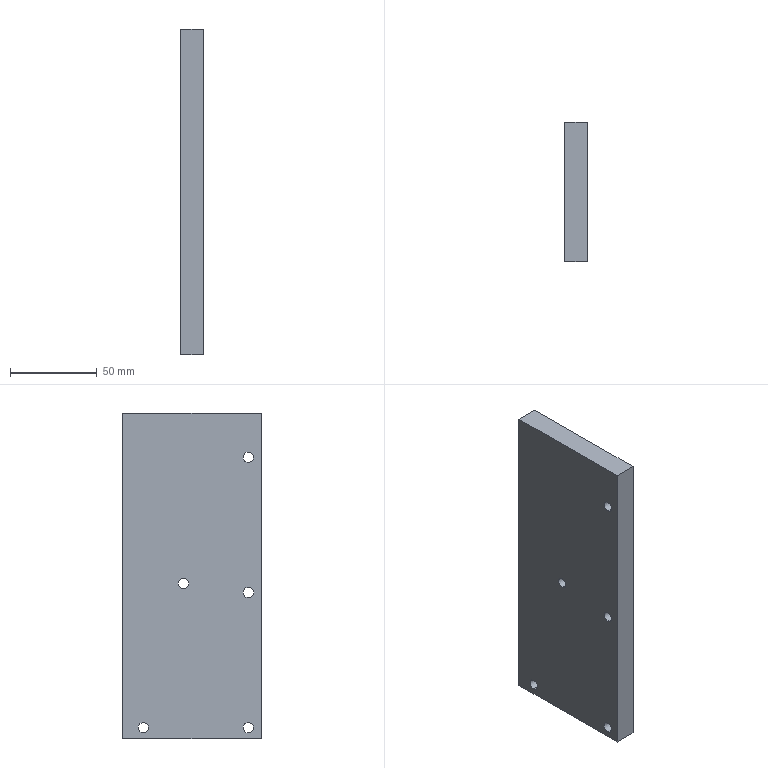Part | SolidWorks | features Cut 6, Extrusion 1 | 1 solid | 31 faces | box 13 x 80 x 188 mm | volume 192174 mm3 | cylinder 20 | plane 11 | commonest cylinder face diameters 6 x10 10 x10
STEP:
#1=CARTESIAN_POINT('',(0.,28.,-84.5));
#2=VERTEX_POINT('',#1);
#3=CARTESIAN_POINT('',(0.,28.,-90.5));
#4=VERTEX_POINT('',#3);
#5=CARTESIAN_POINT('',(0.,28.,-87.5));
#6=DIRECTION('',(1.,0.,0.));
#7=DIRECTION('',(0.,0.,1.));
#8=AXIS2_PLACEMENT_3D('',#5,#6,#7);
#9=CIRCLE('',#8,3.);
#10=EDGE_CURVE('',#2,#4,#9,.T.);
#11=ORIENTED_EDGE('',*,*,#10,.F.);
#12=CARTESIAN_POINT('',(7.,28.,-84.5));
#13=VERTEX_POINT('',#12);
#14=CARTESIAN_POINT('',(-0.001,28.,-84.5));
#15=DIRECTION('',(1.,0.,0.));
#16=VECTOR('',#15,1000.);
#17=LINE('',#14,#16);
#18=EDGE_CURVE('',#2,#13,#17,.T.);
#19=ORIENTED_EDGE('',*,*,#18,.T.);
#20=CARTESIAN_POINT('',(7.,28.,-90.5));
#21=VERTEX_POINT('',#20);
#22=CARTESIAN_POINT('',(7.,28.,-87.5));
#23=DIRECTION('',(-1.,0.,0.));
#24=DIRECTION('',(0.,0.,-1.));
#25=AXIS2_PLACEMENT_3D('',#22,#23,#24);
#26=CIRCLE('',#25,3.);
#27=EDGE_CURVE('',#21,#13,#26,.T.);
#28=ORIENTED_EDGE('',*,*,#27,.F.);
#29=CARTESIAN_POINT('',(-0.001,28.,-90.5));
#30=DIRECTION('',(1.,0.,0.));
#31=VECTOR('',#30,1000.);
#32=LINE('',#29,#31);
#33=EDGE_CURVE('',#4,#21,#32,.T.);
#34=ORIENTED_EDGE('',*,*,#33,.F.);
#35=EDGE_LOOP('',(#11,#19,#28,#34));
#36=FACE_OUTER_BOUND('',#35,.T.);
#37=CARTESIAN_POINT('',(-0.001,28.,-87.5));
#38=DIRECTION('',(1.,0.,0.));
#39=DIRECTION('',(0.,0.,-1.));
#40=AXIS2_PLACEMENT_3D('',#37,#38,#39);
#41=CYLINDRICAL_SURFACE('',#40,3.);
#42=ADVANCED_FACE('',(#36),#41,.F.);
#43=CARTESIAN_POINT('',(7.,28.,-82.5));
#44=VERTEX_POINT('',#43);
#45=CARTESIAN_POINT('',(7.,28.,-92.5));
#46=VERTEX_POINT('',#45);
#47=CARTESIAN_POINT('',(7.,28.,-87.5));
#48=DIRECTION('',(1.,0.,0.));
#49=DIRECTION('',(0.,0.,-1.));
#50=AXIS2_PLACEMENT_3D('',#47,#48,#49);
#51=CIRCLE('',#50,5.);
#52=EDGE_CURVE('',#44,#46,#51,.T.);
#53=ORIENTED_EDGE('',*,*,#52,.F.);
#54=CARTESIAN_POINT('',(13.,28.,-82.5));
#55=VERTEX_POINT('',#54);
#56=CARTESIAN_POINT('',(7.,28.,-82.5));
#57=DIRECTION('',(1.,0.,0.));
#58=VECTOR('',#57,1000.);
#59=LINE('',#56,#58);
#60=EDGE_CURVE('',#44,#55,#59,.T.);
#61=ORIENTED_EDGE('',*,*,#60,.T.);
#62=CARTESIAN_POINT('',(13.,28.,-92.5));
#63=VERTEX_POINT('',#62);
#64=CARTESIAN_POINT('',(13.,28.,-87.5));
#65=DIRECTION('',(1.,0.,0.));
#66=DIRECTION('',(0.,0.,-1.));
#67=AXIS2_PLACEMENT_3D('',#64,#65,#66);
#68=CIRCLE('',#67,5.);
#69=EDGE_CURVE('',#55,#63,#68,.T.);
#70=ORIENTED_EDGE('',*,*,#69,.T.);
#71=CARTESIAN_POINT('',(7.,28.,-92.5));
#72=DIRECTION('',(1.,0.,0.));
#73=VECTOR('',#72,1000.);
#74=LINE('',#71,#73);
#75=EDGE_CURVE('',#46,#63,#74,.T.);
#76=ORIENTED_EDGE('',*,*,#75,.F.);
#77=EDGE_LOOP('',(#53,#61,#70,#76));
#78=FACE_OUTER_BOUND('',#77,.T.);
#79=CARTESIAN_POINT('',(7.,28.,-87.5));
#80=DIRECTION('',(1.,0.,0.));
#81=DIRECTION('',(0.,0.,-1.));
#82=AXIS2_PLACEMENT_3D('',#79,#80,#81);
#83=CYLINDRICAL_SURFACE('',#82,5.);
#84=ADVANCED_FACE('',(#78),#83,.F.);
#85=CARTESIAN_POINT('',(0.,-32.5,-84.5));
#86=VERTEX_POINT('',#85);
#87=CARTESIAN_POINT('',(0.,-32.5,-90.5));
#88=VERTEX_POINT('',#87);
#89=CARTESIAN_POINT('',(0.,-32.5,-87.5));
#90=DIRECTION('',(1.,0.,0.));
#91=DIRECTION('',(0.,0.,1.));
#92=AXIS2_PLACEMENT_3D('',#89,#90,#91);
#93=CIRCLE('',#92,3.);
#94=EDGE_CURVE('',#86,#88,#93,.T.);
#95=ORIENTED_EDGE('',*,*,#94,.F.);
#96=CARTESIAN_POINT('',(7.,-32.5,-84.5));
#97=VERTEX_POINT('',#96);
#98=CARTESIAN_POINT('',(-0.001,-32.5,-84.5));
#99=DIRECTION('',(1.,0.,0.));
#100=VECTOR('',#99,1000.);
#101=LINE('',#98,#100);
#102=EDGE_CURVE('',#86,#97,#101,.T.);
#103=ORIENTED_EDGE('',*,*,#102,.T.);
#104=CARTESIAN_POINT('',(7.,-32.5,-90.5));
#105=VERTEX_POINT('',#104);
#106=CARTESIAN_POINT('',(7.,-32.5,-87.5));
#107=DIRECTION('',(-1.,0.,0.));
#108=DIRECTION('',(0.,0.,-1.));
#109=AXIS2_PLACEMENT_3D('',#106,#107,#108);
#110=CIRCLE('',#109,3.);
#111=EDGE_CURVE('',#105,#97,#110,.T.);
#112=ORIENTED_EDGE('',*,*,#111,.F.);
#113=CARTESIAN_POINT('',(-0.001,-32.5,-90.5));
#114=DIRECTION('',(1.,0.,0.));
#115=VECTOR('',#114,1000.);
#116=LINE('',#113,#115);
#117=EDGE_CURVE('',#88,#105,#116,.T.);
#118=ORIENTED_EDGE('',*,*,#117,.F.);
#119=EDGE_LOOP('',(#95,#103,#112,#118));
#120=FACE_OUTER_BOUND('',#119,.T.);
#121=CARTESIAN_POINT('',(-0.001,-32.5,-87.5));
#122=DIRECTION('',(1.,0.,0.));
#123=DIRECTION('',(0.,0.,-1.));
#124=AXIS2_PLACEMENT_3D('',#121,#122,#123);
#125=CYLINDRICAL_SURFACE('',#124,3.);
#126=ADVANCED_FACE('',(#120),#125,.F.);
#127=CARTESIAN_POINT('',(0.,-32.5,-6.5));
#128=VERTEX_POINT('',#127);
#129=CARTESIAN_POINT('',(0.,-32.5,-12.5));
#130=VERTEX_POINT('',#129);
#131=CARTESIAN_POINT('',(0.,-32.5,-9.5));
#132=DIRECTION('',(1.,0.,0.));
#133=DIRECTION('',(0.,0.,1.));
#134=AXIS2_PLACEMENT_3D('',#131,#132,#133);
#135=CIRCLE('',#134,3.);
#136=EDGE_CURVE('',#128,#130,#135,.T.);
#137=ORIENTED_EDGE('',*,*,#136,.F.);
#138=CARTESIAN_POINT('',(7.,-32.5,-6.5));
#139=VERTEX_POINT('',#138);
#140=CARTESIAN_POINT('',(-0.001,-32.5,-6.5));
#141=DIRECTION('',(1.,0.,0.));
#142=VECTOR('',#141,1000.);
#143=LINE('',#140,#142);
#144=EDGE_CURVE('',#128,#139,#143,.T.);
#145=ORIENTED_EDGE('',*,*,#144,.T.);
#146=CARTESIAN_POINT('',(7.,-32.5,-12.5));
#147=VERTEX_POINT('',#146);
#148=CARTESIAN_POINT('',(7.,-32.5,-9.5));
#149=DIRECTION('',(-1.,0.,0.));
#150=DIRECTION('',(0.,0.,-1.));
#151=AXIS2_PLACEMENT_3D('',#148,#149,#150);
#152=CIRCLE('',#151,3.);
#153=EDGE_CURVE('',#147,#139,#152,.T.);
#154=ORIENTED_EDGE('',*,*,#153,.F.);
#155=CARTESIAN_POINT('',(-0.001,-32.5,-12.5));
#156=DIRECTION('',(1.,0.,0.));
#157=VECTOR('',#156,1000.);
#158=LINE('',#155,#157);
#159=EDGE_CURVE('',#130,#147,#158,.T.);
#160=ORIENTED_EDGE('',*,*,#159,.F.);
#161=EDGE_LOOP('',(#137,#145,#154,#160));
#162=FACE_OUTER_BOUND('',#161,.T.);
#163=CARTESIAN_POINT('',(-0.001,-32.5,-9.5));
#164=DIRECTION('',(1.,0.,0.));
#165=DIRECTION('',(0.,0.,-1.));
#166=AXIS2_PLACEMENT_3D('',#163,#164,#165);
#167=CYLINDRICAL_SURFACE('',#166,3.);
#168=ADVANCED_FACE('',(#162),#167,.F.);
#169=CARTESIAN_POINT('',(0.,-32.5,71.5));
#170=VERTEX_POINT('',#169);
#171=CARTESIAN_POINT('',(0.,-32.5,65.5));
#172=VERTEX_POINT('',#171);
#173=CARTESIAN_POINT('',(0.,-32.5,68.5));
#174=DIRECTION('',(1.,0.,0.));
#175=DIRECTION('',(0.,0.,1.));
#176=AXIS2_PLACEMENT_3D('',#173,#174,#175);
#177=CIRCLE('',#176,3.);
#178=EDGE_CURVE('',#170,#172,#177,.T.);
#179=ORIENTED_EDGE('',*,*,#178,.F.);
#180=CARTESIAN_POINT('',(7.,-32.5,71.5));
#181=VERTEX_POINT('',#180);
#182=CARTESIAN_POINT('',(-0.001,-32.5,71.5));
#183=DIRECTION('',(1.,0.,0.));
#184=VECTOR('',#183,1000.);
#185=LINE('',#182,#184);
#186=EDGE_CURVE('',#170,#181,#185,.T.);
#187=ORIENTED_EDGE('',*,*,#186,.T.);
#188=CARTESIAN_POINT('',(7.,-32.5,65.5));
#189=VERTEX_POINT('',#188);
#190=CARTESIAN_POINT('',(7.,-32.5,68.5));
#191=DIRECTION('',(-1.,0.,0.));
#192=DIRECTION('',(0.,0.,-1.));
#193=AXIS2_PLACEMENT_3D('',#190,#191,#192);
#194=CIRCLE('',#193,3.);
#195=EDGE_CURVE('',#189,#181,#194,.T.);
#196=ORIENTED_EDGE('',*,*,#195,.F.);
#197=CARTESIAN_POINT('',(-0.001,-32.5,65.5));
#198=DIRECTION('',(1.,0.,0.));
#199=VECTOR('',#198,1000.);
#200=LINE('',#197,#199);
#201=EDGE_CURVE('',#172,#189,#200,.T.);
#202=ORIENTED_EDGE('',*,*,#201,.F.);
#203=EDGE_LOOP('',(#179,#187,#196,#202));
#204=FACE_OUTER_BOUND('',#203,.T.);
#205=CARTESIAN_POINT('',(-0.001,-32.5,68.5));
#206=DIRECTION('',(1.,0.,0.));
#207=DIRECTION('',(0.,0.,-1.));
#208=AXIS2_PLACEMENT_3D('',#205,#206,#207);
#209=CYLINDRICAL_SURFACE('',#208,3.);
#210=ADVANCED_FACE('',(#204),#209,.F.);
#211=CARTESIAN_POINT('',(7.,-32.5,-82.5));
#212=VERTEX_POINT('',#211);
#213=CARTESIAN_POINT('',(7.,-32.5,-92.5));
#214=VERTEX_POINT('',#213);
#215=CARTESIAN_POINT('',(7.,-32.5,-87.5));
#216=DIRECTION('',(1.,0.,0.));
#217=DIRECTION('',(0.,0.,-1.));
#218=AXIS2_PLACEMENT_3D('',#215,#216,#217);
#219=CIRCLE('',#218,5.);
#220=EDGE_CURVE('',#212,#214,#219,.T.);
#221=ORIENTED_EDGE('',*,*,#220,.F.);
#222=CARTESIAN_POINT('',(13.,-32.5,-82.5));
#223=VERTEX_POINT('',#222);
#224=CARTESIAN_POINT('',(7.,-32.5,-82.5));
#225=DIRECTION('',(1.,0.,0.));
#226=VECTOR('',#225,1000.);
#227=LINE('',#224,#226);
#228=EDGE_CURVE('',#212,#223,#227,.T.);
#229=ORIENTED_EDGE('',*,*,#228,.T.);
#230=CARTESIAN_POINT('',(13.,-32.5,-92.5));
#231=VERTEX_POINT('',#230);
#232=CARTESIAN_POINT('',(13.,-32.5,-87.5));
#233=DIRECTION('',(1.,0.,0.));
#234=DIRECTION('',(0.,0.,-1.));
#235=AXIS2_PLACEMENT_3D('',#232,#233,#234);
#236=CIRCLE('',#235,5.);
#237=EDGE_CURVE('',#223,#231,#236,.T.);
#238=ORIENTED_EDGE('',*,*,#237,.T.);
#239=CARTESIAN_POINT('',(7.,-32.5,-92.5));
#240=DIRECTION('',(1.,0.,0.));
#241=VECTOR('',#240,1000.);
#242=LINE('',#239,#241);
#243=EDGE_CURVE('',#214,#231,#242,.T.);
#244=ORIENTED_EDGE('',*,*,#243,.F.);
#245=EDGE_LOOP('',(#221,#229,#238,#244));
#246=FACE_OUTER_BOUND('',#245,.T.);
#247=CARTESIAN_POINT('',(7.,-32.5,-87.5));
#248=DIRECTION('',(1.,0.,0.));
#249=DIRECTION('',(0.,0.,-1.));
#250=AXIS2_PLACEMENT_3D('',#247,#248,#249);
#251=CYLINDRICAL_SURFACE('',#250,5.);
#252=ADVANCED_FACE('',(#246),#251,.F.);
#253=CARTESIAN_POINT('',(7.,-32.5,-4.5));
#254=VERTEX_POINT('',#253);
#255=CARTESIAN_POINT('',(7.,-32.5,-14.5));
#256=VERTEX_POINT('',#255);
#257=CARTESIAN_POINT('',(7.,-32.5,-9.5));
#258=DIRECTION('',(1.,0.,0.));
#259=DIRECTION('',(0.,0.,-1.));
#260=AXIS2_PLACEMENT_3D('',#257,#258,#259);
#261=CIRCLE('',#260,5.);
#262=EDGE_CURVE('',#254,#256,#261,.T.);
#263=ORIENTED_EDGE('',*,*,#262,.F.);
#264=CARTESIAN_POINT('',(13.,-32.5,-4.5));
#265=VERTEX_POINT('',#264);
#266=CARTESIAN_POINT('',(7.,-32.5,-4.5));
#267=DIRECTION('',(1.,0.,0.));
#268=VECTOR('',#267,1000.);
#269=LINE('',#266,#268);
#270=EDGE_CURVE('',#254,#265,#269,.T.);
#271=ORIENTED_EDGE('',*,*,#270,.T.);
#272=CARTESIAN_POINT('',(13.,-32.5,-14.5));
#273=VERTEX_POINT('',#272);
#274=CARTESIAN_POINT('',(13.,-32.5,-9.5));
#275=DIRECTION('',(1.,0.,0.));
#276=DIRECTION('',(0.,0.,-1.));
#277=AXIS2_PLACEMENT_3D('',#274,#275,#276);
#278=CIRCLE('',#277,5.);
#279=EDGE_CURVE('',#265,#273,#278,.T.);
#280=ORIENTED_EDGE('',*,*,#279,.T.);
#281=CARTESIAN_POINT('',(7.,-32.5,-14.5));
#282=DIRECTION('',(1.,0.,0.));
#283=VECTOR('',#282,1000.);
#284=LINE('',#281,#283);
#285=EDGE_CURVE('',#256,#273,#284,.T.);
#286=ORIENTED_EDGE('',*,*,#285,.F.);
#287=EDGE_LOOP('',(#263,#271,#280,#286));
#288=FACE_OUTER_BOUND('',#287,.T.);
#289=CARTESIAN_POINT('',(7.,-32.5,-9.5));
#290=DIRECTION('',(1.,0.,0.));
#291=DIRECTION('',(0.,0.,-1.));
#292=AXIS2_PLACEMENT_3D('',#289,#290,#291);
#293=CYLINDRICAL_SURFACE('',#292,5.);
#294=ADVANCED_FACE('',(#288),#293,.F.);
#295=CARTESIAN_POINT('',(7.,-32.5,73.5));
#296=VERTEX_POINT('',#295);
#297=CARTESIAN_POINT('',(7.,-32.5,63.5));
#298=VERTEX_POINT('',#297);
#299=CARTESIAN_POINT('',(7.,-32.5,68.5));
#300=DIRECTION('',(1.,0.,0.));
#301=DIRECTION('',(0.,0.,-1.));
#302=AXIS2_PLACEMENT_3D('',#299,#300,#301);
#303=CIRCLE('',#302,5.);
#304=EDGE_CURVE('',#296,#298,#303,.T.);
#305=ORIENTED_EDGE('',*,*,#304,.F.);
#306=CARTESIAN_POINT('',(13.,-32.5,73.5));
#307=VERTEX_POINT('',#306);
#308=CARTESIAN_POINT('',(7.,-32.5,73.5));
#309=DIRECTION('',(1.,0.,0.));
#310=VECTOR('',#309,1000.);
#311=LINE('',#308,#310);
#312=EDGE_CURVE('',#296,#307,#311,.T.);
#313=ORIENTED_EDGE('',*,*,#312,.T.);
#314=CARTESIAN_POINT('',(13.,-32.5,63.5));
#315=VERTEX_POINT('',#314);
#316=CARTESIAN_POINT('',(13.,-32.5,68.5));
#317=DIRECTION('',(1.,0.,0.));
#318=DIRECTION('',(0.,0.,-1.));
#319=AXIS2_PLACEMENT_3D('',#316,#317,#318);
#320=CIRCLE('',#319,5.);
#321=EDGE_CURVE('',#307,#315,#320,.T.);
#322=ORIENTED_EDGE('',*,*,#321,.T.);
#323=CARTESIAN_POINT('',(7.,-32.5,63.5));
#324=DIRECTION('',(1.,0.,0.));
#325=VECTOR('',#324,1000.);
#326=LINE('',#323,#325);
#327=EDGE_CURVE('',#298,#315,#326,.T.);
#328=ORIENTED_EDGE('',*,*,#327,.F.);
#329=EDGE_LOOP('',(#305,#313,#322,#328));
#330=FACE_OUTER_BOUND('',#329,.T.);
#331=CARTESIAN_POINT('',(7.,-32.5,68.5));
#332=DIRECTION('',(1.,0.,0.));
#333=DIRECTION('',(0.,0.,-1.));
#334=AXIS2_PLACEMENT_3D('',#331,#332,#333);
#335=CYLINDRICAL_SURFACE('',#334,5.);
#336=ADVANCED_FACE('',(#330),#335,.F.);
#337=CARTESIAN_POINT('',(0.,4.893,-1.3));
#338=VERTEX_POINT('',#337);
#339=CARTESIAN_POINT('',(0.,4.893,-7.3));
#340=VERTEX_POINT('',#339);
#341=CARTESIAN_POINT('',(0.,4.893,-4.3));
#342=DIRECTION('',(1.,0.,0.));
#343=DIRECTION('',(0.,0.,1.));
#344=AXIS2_PLACEMENT_3D('',#341,#342,#343);
#345=CIRCLE('',#344,3.);
#346=EDGE_CURVE('',#338,#340,#345,.T.);
#347=ORIENTED_EDGE('',*,*,#346,.F.);
#348=CARTESIAN_POINT('',(7.,4.893,-1.3));
#349=VERTEX_POINT('',#348);
#350=CARTESIAN_POINT('',(-0.001,4.893,-1.3));
#351=DIRECTION('',(1.,0.,0.));
#352=VECTOR('',#351,1000.);
#353=LINE('',#350,#352);
#354=EDGE_CURVE('',#338,#349,#353,.T.);
#355=ORIENTED_EDGE('',*,*,#354,.T.);
#356=CARTESIAN_POINT('',(7.,4.893,-7.3));
#357=VERTEX_POINT('',#356);
#358=CARTESIAN_POINT('',(7.,4.893,-4.3));
#359=DIRECTION('',(-1.,0.,0.));
#360=DIRECTION('',(0.,0.,-1.));
#361=AXIS2_PLACEMENT_3D('',#358,#359,#360);
#362=CIRCLE('',#361,3.);
#363=EDGE_CURVE('',#357,#349,#362,.T.);
#364=ORIENTED_EDGE('',*,*,#363,.F.);
#365=CARTESIAN_POINT('',(-0.001,4.893,-7.3));
#366=DIRECTION('',(1.,0.,0.));
#367=VECTOR('',#366,1000.);
#368=LINE('',#365,#367);
#369=EDGE_CURVE('',#340,#357,#368,.T.);
#370=ORIENTED_EDGE('',*,*,#369,.F.);
#371=EDGE_LOOP('',(#347,#355,#364,#370));
#372=FACE_OUTER_BOUND('',#371,.T.);
#373=CARTESIAN_POINT('',(-0.001,4.893,-4.3));
#374=DIRECTION('',(1.,0.,0.));
#375=DIRECTION('',(0.,0.,-1.));
#376=AXIS2_PLACEMENT_3D('',#373,#374,#375);
#377=CYLINDRICAL_SURFACE('',#376,3.);
#378=ADVANCED_FACE('',(#372),#377,.F.);
#379=CARTESIAN_POINT('',(7.,4.893,0.7));
#380=VERTEX_POINT('',#379);
#381=CARTESIAN_POINT('',(7.,4.893,-9.3));
#382=VERTEX_POINT('',#381);
#383=CARTESIAN_POINT('',(7.,4.893,-4.3));
#384=DIRECTION('',(1.,0.,0.));
#385=DIRECTION('',(0.,0.,-1.));
#386=AXIS2_PLACEMENT_3D('',#383,#384,#385);
#387=CIRCLE('',#386,5.);
#388=EDGE_CURVE('',#380,#382,#387,.T.);
#389=ORIENTED_EDGE('',*,*,#388,.F.);
#390=CARTESIAN_POINT('',(13.,4.893,0.7));
#391=VERTEX_POINT('',#390);
#392=CARTESIAN_POINT('',(7.,4.893,0.7));
#393=DIRECTION('',(1.,0.,0.));
#394=VECTOR('',#393,1000.);
#395=LINE('',#392,#394);
#396=EDGE_CURVE('',#380,#391,#395,.T.);
#397=ORIENTED_EDGE('',*,*,#396,.T.);
#398=CARTESIAN_POINT('',(13.,4.893,-9.3));
#399=VERTEX_POINT('',#398);
#400=CARTESIAN_POINT('',(13.,4.893,-4.3));
#401=DIRECTION('',(1.,0.,0.));
#402=DIRECTION('',(0.,0.,-1.));
#403=AXIS2_PLACEMENT_3D('',#400,#401,#402);
#404=CIRCLE('',#403,5.);
#405=EDGE_CURVE('',#391,#399,#404,.T.);
#406=ORIENTED_EDGE('',*,*,#405,.T.);
#407=CARTESIAN_POINT('',(7.,4.893,-9.3));
#408=DIRECTION('',(1.,0.,0.));
#409=VECTOR('',#408,1000.);
#410=LINE('',#407,#409);
#411=EDGE_CURVE('',#382,#399,#410,.T.);
#412=ORIENTED_EDGE('',*,*,#411,.F.);
#413=EDGE_LOOP('',(#389,#397,#406,#412));
#414=FACE_OUTER_BOUND('',#413,.T.);
#415=CARTESIAN_POINT('',(7.,4.893,-4.3));
#416=DIRECTION('',(1.,0.,0.));
#417=DIRECTION('',(0.,0.,-1.));
#418=AXIS2_PLACEMENT_3D('',#415,#416,#417);
#419=CYLINDRICAL_SURFACE('',#418,5.);
#420=ADVANCED_FACE('',(#414),#419,.F.);
#421=CARTESIAN_POINT('',(0.,-40.,-94.));
#422=VERTEX_POINT('',#421);
#423=CARTESIAN_POINT('',(0.,40.,-94.));
#424=VERTEX_POINT('',#423);
#425=CARTESIAN_POINT('',(0.,-40.,-94.));
#426=DIRECTION('',(0.,1.,0.));
#427=VECTOR('',#426,1000.);
#428=LINE('',#425,#427);
#429=EDGE_CURVE('',#422,#424,#428,.T.);
#430=ORIENTED_EDGE('',*,*,#429,.T.);
#431=CARTESIAN_POINT('',(13.,40.,-94.));
#432=VERTEX_POINT('',#431);
#433=CARTESIAN_POINT('',(13.,40.,-94.));
#434=DIRECTION('',(-1.,0.,0.));
#435=VECTOR('',#434,1000.);
#436=LINE('',#433,#435);
#437=EDGE_CURVE('',#432,#424,#436,.T.);
#438=ORIENTED_EDGE('',*,*,#437,.F.);
#439=CARTESIAN_POINT('',(13.,-40.,-94.));
#440=VERTEX_POINT('',#439);
#441=CARTESIAN_POINT('',(13.,-40.,-94.));
#442=DIRECTION('',(0.,1.,0.));
#443=VECTOR('',#442,1000.);
#444=LINE('',#441,#443);
#445=EDGE_CURVE('',#440,#432,#444,.T.);
#446=ORIENTED_EDGE('',*,*,#445,.F.);
#447=CARTESIAN_POINT('',(13.,-40.,-94.));
#448=DIRECTION('',(-1.,0.,0.));
#449=VECTOR('',#448,1000.);
#450=LINE('',#447,#449);
#451=EDGE_CURVE('',#440,#422,#450,.T.);
#452=ORIENTED_EDGE('',*,*,#451,.T.);
#453=EDGE_LOOP('',(#430,#438,#446,#452));
#454=FACE_OUTER_BOUND('',#453,.T.);
#455=CARTESIAN_POINT('',(13.,-40.,-94.));
#456=DIRECTION('',(0.,0.,1.));
#457=DIRECTION('',(1.,0.,0.));
#458=AXIS2_PLACEMENT_3D('',#455,#456,#457);
#459=PLANE('',#458);
#460=ADVANCED_FACE('',(#454),#459,.F.);
#461=CARTESIAN_POINT('',(0.,40.,94.));
#462=VERTEX_POINT('',#461);
#463=CARTESIAN_POINT('',(0.,40.,94.));
#464=DIRECTION('',(0.,0.,1.));
#465=VECTOR('',#464,1000.);
#466=LINE('',#463,#465);
#467=EDGE_CURVE('',#424,#462,#466,.T.);
#468=ORIENTED_EDGE('',*,*,#467,.T.);
#469=CARTESIAN_POINT('',(13.,40.,94.));
#470=VERTEX_POINT('',#469);
#471=CARTESIAN_POINT('',(13.,40.,94.));
#472=DIRECTION('',(-1.,0.,0.));
#473=VECTOR('',#472,1000.);
#474=LINE('',#471,#473);
#475=EDGE_CURVE('',#470,#462,#474,.T.);
#476=ORIENTED_EDGE('',*,*,#475,.F.);
#477=CARTESIAN_POINT('',(13.,40.,94.));
#478=DIRECTION('',(0.,0.,1.));
#479=VECTOR('',#478,1000.);
#480=LINE('',#477,#479);
#481=EDGE_CURVE('',#432,#470,#480,.T.);
#482=ORIENTED_EDGE('',*,*,#481,.F.);
#483=ORIENTED_EDGE('',*,*,#437,.T.);
#484=EDGE_LOOP('',(#468,#476,#482,#483));
#485=FACE_OUTER_BOUND('',#484,.T.);
#486=CARTESIAN_POINT('',(13.,40.,94.));
#487=DIRECTION('',(0.,-1.,0.));
#488=DIRECTION('',(0.,0.,-1.));
#489=AXIS2_PLACEMENT_3D('',#486,#487,#488);
#490=PLANE('',#489);
#491=ADVANCED_FACE('',(#485),#490,.F.);
#492=CARTESIAN_POINT('',(0.,-40.,94.));
#493=VERTEX_POINT('',#492);
#494=CARTESIAN_POINT('',(0.,-40.,94.));
#495=DIRECTION('',(0.,-1.,0.));
#496=VECTOR('',#495,1000.);
#497=LINE('',#494,#496);
#498=EDGE_CURVE('',#462,#493,#497,.T.);
#499=ORIENTED_EDGE('',*,*,#498,.T.);
#500=CARTESIAN_POINT('',(13.,-40.,94.));
#501=VERTEX_POINT('',#500);
#502=CARTESIAN_POINT('',(13.,-40.,94.));
#503=DIRECTION('',(-1.,0.,0.));
#504=VECTOR('',#503,1000.);
#505=LINE('',#502,#504);
#506=EDGE_CURVE('',#501,#493,#505,.T.);
#507=ORIENTED_EDGE('',*,*,#506,.F.);
#508=CARTESIAN_POINT('',(13.,-40.,94.));
#509=DIRECTION('',(0.,-1.,0.));
#510=VECTOR('',#509,1000.);
#511=LINE('',#508,#510);
#512=EDGE_CURVE('',#470,#501,#511,.T.);
#513=ORIENTED_EDGE('',*,*,#512,.F.);
#514=ORIENTED_EDGE('',*,*,#475,.T.);
#515=EDGE_LOOP('',(#499,#507,#513,#514));
#516=FACE_OUTER_BOUND('',#515,.T.);
#517=CARTESIAN_POINT('',(13.,-40.,94.));
#518=DIRECTION('',(0.,0.,-1.));
#519=DIRECTION('',(-1.,0.,0.));
#520=AXIS2_PLACEMENT_3D('',#517,#518,#519);
#521=PLANE('',#520);
#522=ADVANCED_FACE('',(#516),#521,.F.);
#523=CARTESIAN_POINT('',(0.,-40.,94.));
#524=DIRECTION('',(0.,0.,-1.));
#525=VECTOR('',#524,1000.);
#526=LINE('',#523,#525);
#527=EDGE_CURVE('',#493,#422,#526,.T.);
#528=ORIENTED_EDGE('',*,*,#527,.T.);
#529=ORIENTED_EDGE('',*,*,#451,.F.);
#530=CARTESIAN_POINT('',(13.,-40.,94.));
#531=DIRECTION('',(0.,0.,-1.));
#532=VECTOR('',#531,1000.);
#533=LINE('',#530,#532);
#534=EDGE_CURVE('',#501,#440,#533,.T.);
#535=ORIENTED_EDGE('',*,*,#534,.F.);
#536=ORIENTED_EDGE('',*,*,#506,.T.);
#537=EDGE_LOOP('',(#528,#529,#535,#536));
#538=FACE_OUTER_BOUND('',#537,.T.);
#539=CARTESIAN_POINT('',(13.,-40.,94.));
#540=DIRECTION('',(0.,1.,0.));
#541=DIRECTION('',(0.,0.,1.));
#542=AXIS2_PLACEMENT_3D('',#539,#540,#541);
#543=PLANE('',#542);
#544=ADVANCED_FACE('',(#538),#543,.F.);
#545=CARTESIAN_POINT('',(13.,28.,-87.5));
#546=DIRECTION('',(1.,0.,0.));
#547=DIRECTION('',(0.,0.,-1.));
#548=AXIS2_PLACEMENT_3D('',#545,#546,#547);
#549=CIRCLE('',#548,5.);
#550=EDGE_CURVE('',#63,#55,#549,.T.);
#551=ORIENTED_EDGE('',*,*,#550,.F.);
#552=ORIENTED_EDGE('',*,*,#69,.F.);
#553=EDGE_LOOP('',(#551,#552));
#554=FACE_BOUND('',#553,.T.);
#555=CARTESIAN_POINT('',(13.,-32.5,-87.5));
#556=DIRECTION('',(1.,0.,0.));
#557=DIRECTION('',(0.,0.,-1.));
#558=AXIS2_PLACEMENT_3D('',#555,#556,#557);
#559=CIRCLE('',#558,5.);
#560=EDGE_CURVE('',#231,#223,#559,.T.);
#561=ORIENTED_EDGE('',*,*,#560,.F.);
#562=ORIENTED_EDGE('',*,*,#237,.F.);
#563=EDGE_LOOP('',(#561,#562));
#564=FACE_BOUND('',#563,.T.);
#565=CARTESIAN_POINT('',(13.,-32.5,-9.5));
#566=DIRECTION('',(1.,0.,0.));
#567=DIRECTION('',(0.,0.,-1.));
#568=AXIS2_PLACEMENT_3D('',#565,#566,#567);
#569=CIRCLE('',#568,5.);
#570=EDGE_CURVE('',#273,#265,#569,.T.);
#571=ORIENTED_EDGE('',*,*,#570,.F.);
#572=ORIENTED_EDGE('',*,*,#279,.F.);
#573=EDGE_LOOP('',(#571,#572));
#574=FACE_BOUND('',#573,.T.);
#575=CARTESIAN_POINT('',(13.,-32.5,68.5));
#576=DIRECTION('',(1.,0.,0.));
#577=DIRECTION('',(0.,0.,-1.));
#578=AXIS2_PLACEMENT_3D('',#575,#576,#577);
#579=CIRCLE('',#578,5.);
#580=EDGE_CURVE('',#315,#307,#579,.T.);
#581=ORIENTED_EDGE('',*,*,#580,.F.);
#582=ORIENTED_EDGE('',*,*,#321,.F.);
#583=EDGE_LOOP('',(#581,#582));
#584=FACE_BOUND('',#583,.T.);
#585=CARTESIAN_POINT('',(13.,4.893,-4.3));
#586=DIRECTION('',(1.,0.,0.));
#587=DIRECTION('',(0.,0.,-1.));
#588=AXIS2_PLACEMENT_3D('',#585,#586,#587);
#589=CIRCLE('',#588,5.);
#590=EDGE_CURVE('',#399,#391,#589,.T.);
#591=ORIENTED_EDGE('',*,*,#590,.F.);
#592=ORIENTED_EDGE('',*,*,#405,.F.);
#593=EDGE_LOOP('',(#591,#592));
#594=FACE_BOUND('',#593,.T.);
#595=ORIENTED_EDGE('',*,*,#445,.T.);
#596=ORIENTED_EDGE('',*,*,#481,.T.);
#597=ORIENTED_EDGE('',*,*,#512,.T.);
#598=ORIENTED_EDGE('',*,*,#534,.T.);
#599=EDGE_LOOP('',(#595,#596,#597,#598));
#600=FACE_OUTER_BOUND('',#599,.T.);
#601=CARTESIAN_POINT('',(13.,0.,0.));
#602=DIRECTION('',(-1.,0.,0.));
#603=DIRECTION('',(0.,0.,1.));
#604=AXIS2_PLACEMENT_3D('',#601,#602,#603);
#605=PLANE('',#604);
#606=ADVANCED_FACE('',(#554,#564,#574,#584,#594,#600),#605,.F.);
#607=CARTESIAN_POINT('',(0.,28.,-87.5));
#608=DIRECTION('',(1.,0.,0.));
#609=DIRECTION('',(0.,0.,1.));
#610=AXIS2_PLACEMENT_3D('',#607,#608,#609);
#611=CIRCLE('',#610,3.);
#612=EDGE_CURVE('',#4,#2,#611,.T.);
#613=ORIENTED_EDGE('',*,*,#612,.T.);
#614=ORIENTED_EDGE('',*,*,#10,.T.);
#615=EDGE_LOOP('',(#613,#614));
#616=FACE_BOUND('',#615,.T.);
#617=CARTESIAN_POINT('',(0.,-32.5,-87.5));
#618=DIRECTION('',(1.,0.,0.));
#619=DIRECTION('',(0.,0.,1.));
#620=AXIS2_PLACEMENT_3D('',#617,#618,#619);
#621=CIRCLE('',#620,3.);
#622=EDGE_CURVE('',#88,#86,#621,.T.);
#623=ORIENTED_EDGE('',*,*,#622,.T.);
#624=ORIENTED_EDGE('',*,*,#94,.T.);
#625=EDGE_LOOP('',(#623,#624));
#626=FACE_BOUND('',#625,.T.);
#627=CARTESIAN_POINT('',(0.,-32.5,-9.5));
#628=DIRECTION('',(1.,0.,0.));
#629=DIRECTION('',(0.,0.,1.));
#630=AXIS2_PLACEMENT_3D('',#627,#628,#629);
#631=CIRCLE('',#630,3.);
#632=EDGE_CURVE('',#130,#128,#631,.T.);
#633=ORIENTED_EDGE('',*,*,#632,.T.);
#634=ORIENTED_EDGE('',*,*,#136,.T.);
#635=EDGE_LOOP('',(#633,#634));
#636=FACE_BOUND('',#635,.T.);
#637=CARTESIAN_POINT('',(0.,-32.5,68.5));
#638=DIRECTION('',(1.,0.,0.));
#639=DIRECTION('',(0.,0.,1.));
#640=AXIS2_PLACEMENT_3D('',#637,#638,#639);
#641=CIRCLE('',#640,3.);
#642=EDGE_CURVE('',#172,#170,#641,.T.);
#643=ORIENTED_EDGE('',*,*,#642,.T.);
#644=ORIENTED_EDGE('',*,*,#178,.T.);
#645=EDGE_LOOP('',(#643,#644));
#646=FACE_BOUND('',#645,.T.);
#647=CARTESIAN_POINT('',(0.,4.893,-4.3));
#648=DIRECTION('',(1.,0.,0.));
#649=DIRECTION('',(0.,0.,1.));
#650=AXIS2_PLACEMENT_3D('',#647,#648,#649);
#651=CIRCLE('',#650,3.);
#652=EDGE_CURVE('',#340,#338,#651,.T.);
#653=ORIENTED_EDGE('',*,*,#652,.T.);
#654=ORIENTED_EDGE('',*,*,#346,.T.);
#655=EDGE_LOOP('',(#653,#654));
#656=FACE_BOUND('',#655,.T.);
#657=ORIENTED_EDGE('',*,*,#429,.F.);
#658=ORIENTED_EDGE('',*,*,#527,.F.);
#659=ORIENTED_EDGE('',*,*,#498,.F.);
#660=ORIENTED_EDGE('',*,*,#467,.F.);
#661=EDGE_LOOP('',(#657,#658,#659,#660));
#662=FACE_OUTER_BOUND('',#661,.T.);
#663=CARTESIAN_POINT('',(0.,0.,0.));
#664=DIRECTION('',(-1.,0.,0.));
#665=DIRECTION('',(0.,0.,1.));
#666=AXIS2_PLACEMENT_3D('',#663,#664,#665);
#667=PLANE('',#666);
#668=ADVANCED_FACE('',(#616,#626,#636,#646,#656,#662),#667,.T.);
#669=ORIENTED_EDGE('',*,*,#396,.F.);
#670=CARTESIAN_POINT('',(7.,4.893,-4.3));
#671=DIRECTION('',(1.,0.,0.));
#672=DIRECTION('',(0.,0.,-1.));
#673=AXIS2_PLACEMENT_3D('',#670,#671,#672);
#674=CIRCLE('',#673,5.);
#675=EDGE_CURVE('',#382,#380,#674,.T.);
#676=ORIENTED_EDGE('',*,*,#675,.F.);
#677=ORIENTED_EDGE('',*,*,#411,.T.);
#678=ORIENTED_EDGE('',*,*,#590,.T.);
#679=EDGE_LOOP('',(#669,#676,#677,#678));
#680=FACE_OUTER_BOUND('',#679,.T.);
#681=CARTESIAN_POINT('',(7.,4.893,-4.3));
#682=DIRECTION('',(1.,0.,0.));
#683=DIRECTION('',(0.,0.,-1.));
#684=AXIS2_PLACEMENT_3D('',#681,#682,#683);
#685=CYLINDRICAL_SURFACE('',#684,5.);
#686=ADVANCED_FACE('',(#680),#685,.F.);
#687=ORIENTED_EDGE('',*,*,#363,.T.);
#688=CARTESIAN_POINT('',(7.,4.893,-4.3));
#689=DIRECTION('',(-1.,0.,0.));
#690=DIRECTION('',(0.,0.,-1.));
#691=AXIS2_PLACEMENT_3D('',#688,#689,#690);
#692=CIRCLE('',#691,3.);
#693=EDGE_CURVE('',#349,#357,#692,.T.);
#694=ORIENTED_EDGE('',*,*,#693,.T.);
#695=EDGE_LOOP('',(#687,#694));
#696=FACE_BOUND('',#695,.T.);
#697=ORIENTED_EDGE('',*,*,#675,.T.);
#698=ORIENTED_EDGE('',*,*,#388,.T.);
#699=EDGE_LOOP('',(#697,#698));
#700=FACE_OUTER_BOUND('',#699,.T.);
#701=CARTESIAN_POINT('',(7.,0.,0.));
#702=DIRECTION('',(1.,0.,0.));
#703=DIRECTION('',(0.,0.,-1.));
#704=AXIS2_PLACEMENT_3D('',#701,#702,#703);
#705=PLANE('',#704);
#706=ADVANCED_FACE('',(#696,#700),#705,.T.);
#707=ORIENTED_EDGE('',*,*,#354,.F.);
#708=ORIENTED_EDGE('',*,*,#652,.F.);
#709=ORIENTED_EDGE('',*,*,#369,.T.);
#710=ORIENTED_EDGE('',*,*,#693,.F.);
#711=EDGE_LOOP('',(#707,#708,#709,#710));
#712=FACE_OUTER_BOUND('',#711,.T.);
#713=CARTESIAN_POINT('',(-0.001,4.893,-4.3));
#714=DIRECTION('',(1.,0.,0.));
#715=DIRECTION('',(0.,0.,-1.));
#716=AXIS2_PLACEMENT_3D('',#713,#714,#715);
#717=CYLINDRICAL_SURFACE('',#716,3.);
#718=ADVANCED_FACE('',(#712),#717,.F.);
#719=ORIENTED_EDGE('',*,*,#312,.F.);
#720=CARTESIAN_POINT('',(7.,-32.5,68.5));
#721=DIRECTION('',(1.,0.,0.));
#722=DIRECTION('',(0.,0.,-1.));
#723=AXIS2_PLACEMENT_3D('',#720,#721,#722);
#724=CIRCLE('',#723,5.);
#725=EDGE_CURVE('',#298,#296,#724,.T.);
#726=ORIENTED_EDGE('',*,*,#725,.F.);
#727=ORIENTED_EDGE('',*,*,#327,.T.);
#728=ORIENTED_EDGE('',*,*,#580,.T.);
#729=EDGE_LOOP('',(#719,#726,#727,#728));
#730=FACE_OUTER_BOUND('',#729,.T.);
#731=CARTESIAN_POINT('',(7.,-32.5,68.5));
#732=DIRECTION('',(1.,0.,0.));
#733=DIRECTION('',(0.,0.,-1.));
#734=AXIS2_PLACEMENT_3D('',#731,#732,#733);
#735=CYLINDRICAL_SURFACE('',#734,5.);
#736=ADVANCED_FACE('',(#730),#735,.F.);
#737=ORIENTED_EDGE('',*,*,#195,.T.);
#738=CARTESIAN_POINT('',(7.,-32.5,68.5));
#739=DIRECTION('',(-1.,0.,0.));
#740=DIRECTION('',(0.,0.,-1.));
#741=AXIS2_PLACEMENT_3D('',#738,#739,#740);
#742=CIRCLE('',#741,3.);
#743=EDGE_CURVE('',#181,#189,#742,.T.);
#744=ORIENTED_EDGE('',*,*,#743,.T.);
#745=EDGE_LOOP('',(#737,#744));
#746=FACE_BOUND('',#745,.T.);
#747=ORIENTED_EDGE('',*,*,#725,.T.);
#748=ORIENTED_EDGE('',*,*,#304,.T.);
#749=EDGE_LOOP('',(#747,#748));
#750=FACE_OUTER_BOUND('',#749,.T.);
#751=CARTESIAN_POINT('',(7.,0.,0.));
#752=DIRECTION('',(1.,0.,0.));
#753=DIRECTION('',(0.,0.,-1.));
#754=AXIS2_PLACEMENT_3D('',#751,#752,#753);
#755=PLANE('',#754);
#756=ADVANCED_FACE('',(#746,#750),#755,.T.);
#757=ORIENTED_EDGE('',*,*,#270,.F.);
#758=CARTESIAN_POINT('',(7.,-32.5,-9.5));
#759=DIRECTION('',(1.,0.,0.));
#760=DIRECTION('',(0.,0.,-1.));
#761=AXIS2_PLACEMENT_3D('',#758,#759,#760);
#762=CIRCLE('',#761,5.);
#763=EDGE_CURVE('',#256,#254,#762,.T.);
#764=ORIENTED_EDGE('',*,*,#763,.F.);
#765=ORIENTED_EDGE('',*,*,#285,.T.);
#766=ORIENTED_EDGE('',*,*,#570,.T.);
#767=EDGE_LOOP('',(#757,#764,#765,#766));
#768=FACE_OUTER_BOUND('',#767,.T.);
#769=CARTESIAN_POINT('',(7.,-32.5,-9.5));
#770=DIRECTION('',(1.,0.,0.));
#771=DIRECTION('',(0.,0.,-1.));
#772=AXIS2_PLACEMENT_3D('',#769,#770,#771);
#773=CYLINDRICAL_SURFACE('',#772,5.);
#774=ADVANCED_FACE('',(#768),#773,.F.);
#775=ORIENTED_EDGE('',*,*,#153,.T.);
#776=CARTESIAN_POINT('',(7.,-32.5,-9.5));
#777=DIRECTION('',(-1.,0.,0.));
#778=DIRECTION('',(0.,0.,-1.));
#779=AXIS2_PLACEMENT_3D('',#776,#777,#778);
#780=CIRCLE('',#779,3.);
#781=EDGE_CURVE('',#139,#147,#780,.T.);
#782=ORIENTED_EDGE('',*,*,#781,.T.);
#783=EDGE_LOOP('',(#775,#782));
#784=FACE_BOUND('',#783,.T.);
#785=ORIENTED_EDGE('',*,*,#763,.T.);
#786=ORIENTED_EDGE('',*,*,#262,.T.);
#787=EDGE_LOOP('',(#785,#786));
#788=FACE_OUTER_BOUND('',#787,.T.);
#789=CARTESIAN_POINT('',(7.,0.,0.));
#790=DIRECTION('',(1.,0.,0.));
#791=DIRECTION('',(0.,0.,-1.));
#792=AXIS2_PLACEMENT_3D('',#789,#790,#791);
#793=PLANE('',#792);
#794=ADVANCED_FACE('',(#784,#788),#793,.T.);
#795=ORIENTED_EDGE('',*,*,#228,.F.);
#796=CARTESIAN_POINT('',(7.,-32.5,-87.5));
#797=DIRECTION('',(1.,0.,0.));
#798=DIRECTION('',(0.,0.,-1.));
#799=AXIS2_PLACEMENT_3D('',#796,#797,#798);
#800=CIRCLE('',#799,5.);
#801=EDGE_CURVE('',#214,#212,#800,.T.);
#802=ORIENTED_EDGE('',*,*,#801,.F.);
#803=ORIENTED_EDGE('',*,*,#243,.T.);
#804=ORIENTED_EDGE('',*,*,#560,.T.);
#805=EDGE_LOOP('',(#795,#802,#803,#804));
#806=FACE_OUTER_BOUND('',#805,.T.);
#807=CARTESIAN_POINT('',(7.,-32.5,-87.5));
#808=DIRECTION('',(1.,0.,0.));
#809=DIRECTION('',(0.,0.,-1.));
#810=AXIS2_PLACEMENT_3D('',#807,#808,#809);
#811=CYLINDRICAL_SURFACE('',#810,5.);
#812=ADVANCED_FACE('',(#806),#811,.F.);
#813=ORIENTED_EDGE('',*,*,#111,.T.);
#814=CARTESIAN_POINT('',(7.,-32.5,-87.5));
#815=DIRECTION('',(-1.,0.,0.));
#816=DIRECTION('',(0.,0.,-1.));
#817=AXIS2_PLACEMENT_3D('',#814,#815,#816);
#818=CIRCLE('',#817,3.);
#819=EDGE_CURVE('',#97,#105,#818,.T.);
#820=ORIENTED_EDGE('',*,*,#819,.T.);
#821=EDGE_LOOP('',(#813,#820));
#822=FACE_BOUND('',#821,.T.);
#823=ORIENTED_EDGE('',*,*,#801,.T.);
#824=ORIENTED_EDGE('',*,*,#220,.T.);
#825=EDGE_LOOP('',(#823,#824));
#826=FACE_OUTER_BOUND('',#825,.T.);
#827=CARTESIAN_POINT('',(7.,0.,0.));
#828=DIRECTION('',(1.,0.,0.));
#829=DIRECTION('',(0.,0.,-1.));
#830=AXIS2_PLACEMENT_3D('',#827,#828,#829);
#831=PLANE('',#830);
#832=ADVANCED_FACE('',(#822,#826),#831,.T.);
#833=ORIENTED_EDGE('',*,*,#186,.F.);
#834=ORIENTED_EDGE('',*,*,#642,.F.);
#835=ORIENTED_EDGE('',*,*,#201,.T.);
#836=ORIENTED_EDGE('',*,*,#743,.F.);
#837=EDGE_LOOP('',(#833,#834,#835,#836));
#838=FACE_OUTER_BOUND('',#837,.T.);
#839=CARTESIAN_POINT('',(-0.001,-32.5,68.5));
#840=DIRECTION('',(1.,0.,0.));
#841=DIRECTION('',(0.,0.,-1.));
#842=AXIS2_PLACEMENT_3D('',#839,#840,#841);
#843=CYLINDRICAL_SURFACE('',#842,3.);
#844=ADVANCED_FACE('',(#838),#843,.F.);
#845=ORIENTED_EDGE('',*,*,#144,.F.);
#846=ORIENTED_EDGE('',*,*,#632,.F.);
#847=ORIENTED_EDGE('',*,*,#159,.T.);
#848=ORIENTED_EDGE('',*,*,#781,.F.);
#849=EDGE_LOOP('',(#845,#846,#847,#848));
#850=FACE_OUTER_BOUND('',#849,.T.);
#851=CARTESIAN_POINT('',(-0.001,-32.5,-9.5));
#852=DIRECTION('',(1.,0.,0.));
#853=DIRECTION('',(0.,0.,-1.));
#854=AXIS2_PLACEMENT_3D('',#851,#852,#853);
#855=CYLINDRICAL_SURFACE('',#854,3.);
#856=ADVANCED_FACE('',(#850),#855,.F.);
#857=ORIENTED_EDGE('',*,*,#102,.F.);
#858=ORIENTED_EDGE('',*,*,#622,.F.);
#859=ORIENTED_EDGE('',*,*,#117,.T.);
#860=ORIENTED_EDGE('',*,*,#819,.F.);
#861=EDGE_LOOP('',(#857,#858,#859,#860));
#862=FACE_OUTER_BOUND('',#861,.T.);
#863=CARTESIAN_POINT('',(-0.001,-32.5,-87.5));
#864=DIRECTION('',(1.,0.,0.));
#865=DIRECTION('',(0.,0.,-1.));
#866=AXIS2_PLACEMENT_3D('',#863,#864,#865);
#867=CYLINDRICAL_SURFACE('',#866,3.);
#868=ADVANCED_FACE('',(#862),#867,.F.);
#869=ORIENTED_EDGE('',*,*,#60,.F.);
#870=CARTESIAN_POINT('',(7.,28.,-87.5));
#871=DIRECTION('',(1.,0.,0.));
#872=DIRECTION('',(0.,0.,-1.));
#873=AXIS2_PLACEMENT_3D('',#870,#871,#872);
#874=CIRCLE('',#873,5.);
#875=EDGE_CURVE('',#46,#44,#874,.T.);
#876=ORIENTED_EDGE('',*,*,#875,.F.);
#877=ORIENTED_EDGE('',*,*,#75,.T.);
#878=ORIENTED_EDGE('',*,*,#550,.T.);
#879=EDGE_LOOP('',(#869,#876,#877,#878));
#880=FACE_OUTER_BOUND('',#879,.T.);
#881=CARTESIAN_POINT('',(7.,28.,-87.5));
#882=DIRECTION('',(1.,0.,0.));
#883=DIRECTION('',(0.,0.,-1.));
#884=AXIS2_PLACEMENT_3D('',#881,#882,#883);
#885=CYLINDRICAL_SURFACE('',#884,5.);
#886=ADVANCED_FACE('',(#880),#885,.F.);
#887=ORIENTED_EDGE('',*,*,#27,.T.);
#888=CARTESIAN_POINT('',(7.,28.,-87.5));
#889=DIRECTION('',(-1.,0.,0.));
#890=DIRECTION('',(0.,0.,-1.));
#891=AXIS2_PLACEMENT_3D('',#888,#889,#890);
#892=CIRCLE('',#891,3.);
#893=EDGE_CURVE('',#13,#21,#892,.T.);
#894=ORIENTED_EDGE('',*,*,#893,.T.);
#895=EDGE_LOOP('',(#887,#894));
#896=FACE_BOUND('',#895,.T.);
#897=ORIENTED_EDGE('',*,*,#875,.T.);
#898=ORIENTED_EDGE('',*,*,#52,.T.);
#899=EDGE_LOOP('',(#897,#898));
#900=FACE_OUTER_BOUND('',#899,.T.);
#901=CARTESIAN_POINT('',(7.,0.,0.));
#902=DIRECTION('',(1.,0.,0.));
#903=DIRECTION('',(0.,0.,-1.));
#904=AXIS2_PLACEMENT_3D('',#901,#902,#903);
#905=PLANE('',#904);
#906=ADVANCED_FACE('',(#896,#900),#905,.T.);
#907=ORIENTED_EDGE('',*,*,#18,.F.);
#908=ORIENTED_EDGE('',*,*,#612,.F.);
#909=ORIENTED_EDGE('',*,*,#33,.T.);
#910=ORIENTED_EDGE('',*,*,#893,.F.);
#911=EDGE_LOOP('',(#907,#908,#909,#910));
#912=FACE_OUTER_BOUND('',#911,.T.);
#913=CARTESIAN_POINT('',(-0.001,28.,-87.5));
#914=DIRECTION('',(1.,0.,0.));
#915=DIRECTION('',(0.,0.,-1.));
#916=AXIS2_PLACEMENT_3D('',#913,#914,#915);
#917=CYLINDRICAL_SURFACE('',#916,3.);
#918=ADVANCED_FACE('',(#912),#917,.F.);
#919=CLOSED_SHELL('',(#42,#84,#126,#168,#210,#252,#294,#336,#378,#420,#460,#491,#522,#544,#606,#668,#686,#706,#718,#736,#756,#774,#794,#812,#832,#844,#856,#868,#886,#906,#918));
#920=MANIFOLD_SOLID_BREP('',#919);
#921=CARTESIAN_POINT('',(0.,0.,0.));
#922=DIRECTION('',(0.,0.,1.));
#923=DIRECTION('',(1.,0.,0.));
#924=AXIS2_PLACEMENT_3D('',#921,#922,#923);
#925=(LENGTH_UNIT()NAMED_UNIT(*)SI_UNIT(.MILLI.,.METRE.));
#926=UNCERTAINTY_MEASURE_WITH_UNIT(LENGTH_MEASURE(0.00001),#925,'','');
#927=(NAMED_UNIT(*)PLANE_ANGLE_UNIT()SI_UNIT($,.RADIAN.));
#928=(NAMED_UNIT(*)SI_UNIT($,.STERADIAN.)SOLID_ANGLE_UNIT());
#929=(GEOMETRIC_REPRESENTATION_CONTEXT(3)GLOBAL_UNCERTAINTY_ASSIGNED_CONTEXT((#926))GLOBAL_UNIT_ASSIGNED_CONTEXT((#925,#927,#928))REPRESENTATION_CONTEXT('',''));
#930=ADVANCED_BREP_SHAPE_REPRESENTATION('',(#920,#924),#929);